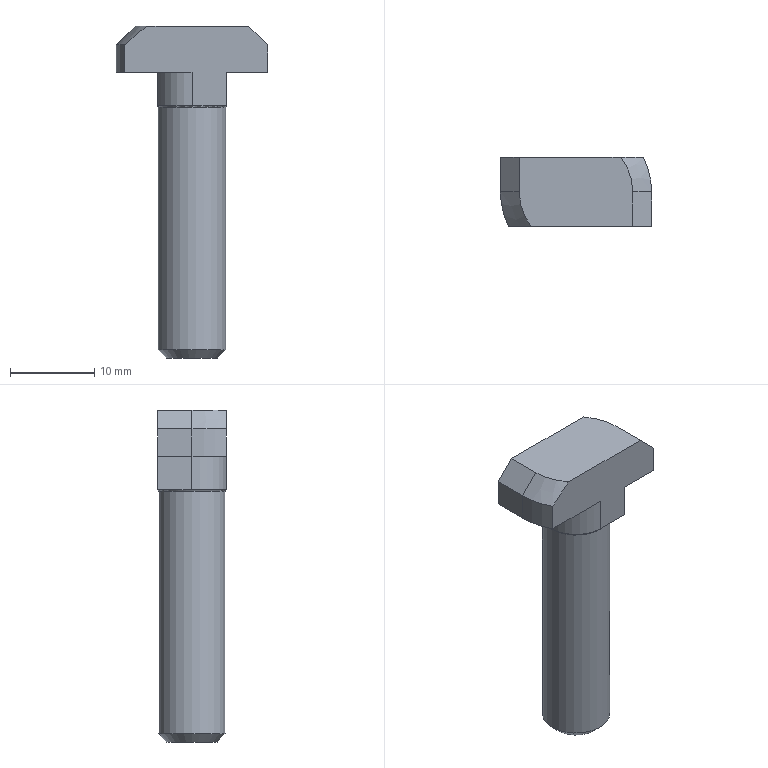Part | STEP file | Left | 1 solid | 25 faces | box 18 x 8.32 x 39.5 mm | volume 2491 mm3 | plane 16 | cylinder 5 | cone 3 | torus 1 | commonest cylinder face diameters 8.2 x2 18 x2 8 x1